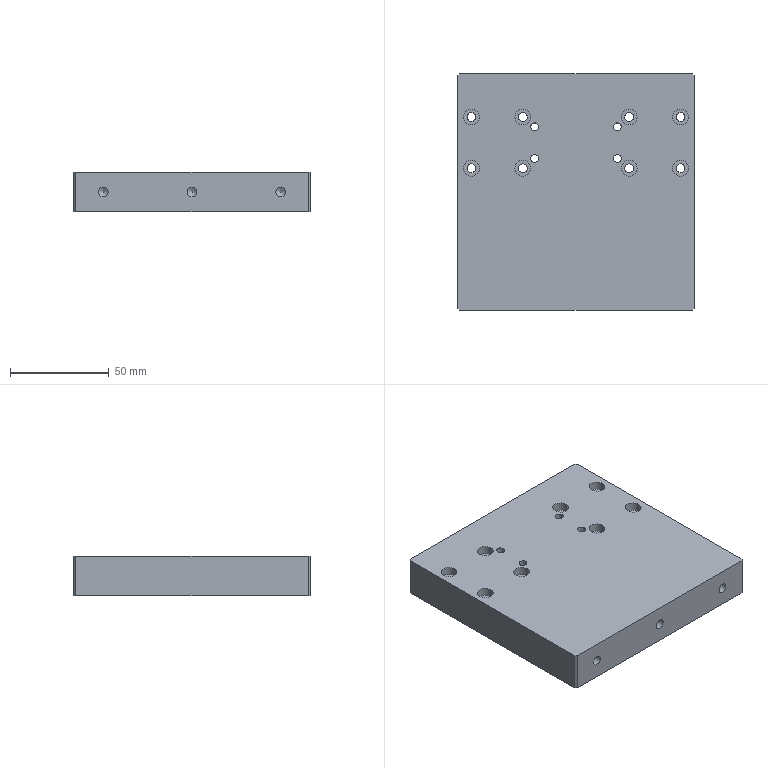CAM job | NX | 3-axis milling, drilling | part box 120 x 120 x 20 mm | stock box 125 x 120 x 25 mm
Tools:
number,name,description,diameter,corner_radius,flute_length,length,flutes
4,D4,平底铣刀-粗,4.0,0.0,25.0,75.0,2
9,D10,平底铣刀-粗,10.0,0.0,35.0,75.0,2
11,D4-J,平底铣刀-精,4.0,0.0,50.0,75.0,2
10,D10-J,平底铣刀-精,10.0,0.0,35.0,75.0,2
1,D80R0.8飞刀,圆鼻刀-粗,80.0,0.8,50.0,75.0,2
1,D80R0.8飞刀-J,圆鼻刀-精,80.0,0.8,50.0,75.0,2
2,D6倒角刀,倒角刀,6.0,0.0,3.0,25.0,2
18,D4铰刀,Drilling Tool,4.0,0.0,75.0,100.0,6
11,ZT4.5,钻头,4.5,0.0,35.0,50.0,2
17,ZT3.9,Drilling Tool,3.9,0.0,35.0,50.0,2
Operations:
program,operation,operation_type,tool,method,geometry_group,spindle_rpm,surface_speed,feed_per_tooth,feed_cut,feed_plunge,cut_length_mm,path_length_mm,cut_time_min,machine_time_min
B,BOTTOM_WALL_FLY_ROUGH_COPY,VolumeBased25DMillingOperation,D80R0.8飞刀,LAYERED_ROUGH-DEPTHK-STEPG,W-B,2800.0,703.696,0.5357,3000.0,100.0,4377.187,4987.758,1.459,1.52
B,BOTTOM_WALL_FLY_FINISH_COPY,VolumeBased25DMillingOperation,D80R0.8飞刀-J,SIDE_FINISH-DEPTHK-STEPG,W-B,4000.0,1005.28,0.125,1000.0,100.0,679.584,775.584,0.6796,0.6892
B,DRILL_CHAMFER_2,Operation,D6倒角刀,METHOD,W-B,8000.0,150.796,0.0625,1000.0,0.0,21.2,226.065,0.0212,0.0417
B,DRILL_CHAMFER_3,Operation,D6倒角刀,METHOD,W-B,8000.0,150.796,0.0625,1000.0,0.0,44.4,420.918,0.0444,0.0821
B,PLANAR_DEBURR_6X45L_COPY,SurfaceContour,D6倒角刀,CLIMB_CHAMFER-DEPTH0-STEPG,W-B,6500.0,122.519,0.1154,1500.0,100.0,622.57,1155.001,0.415,0.4683
A,TOP_FACE,FaceMilling,D80R0.8飞刀,SIDE_FINISH-DEPTHK-STEPG,W-A,4500.0,1385.0,0.1667,1500.0,100.0,714.0,810.0,0.476,0.4856
A,PROFILE_ROUGH_2,VolumeBased25DMillingOperation,D10,METHOD,W-A,8000.0,251.327,0.375,6000.0,80.0,13763.445,13881.945,2.294,2.306
A,SPOT,Operation,D6倒角刀,METHOD,W-A,8000.0,150.796,0.1562,2500.0,0.0,30.0,392.311,0.012,0.0482
A,DRILL,Operation,ZT3.9,METHOD,W-A,3800.0,46.558,0.0395,300.0,0.0,100.503,378.081,0.335,0.3628
A,DRILL_2,Operation,ZT4.5,METHOD,W-A,3800.0,53.721,0.0395,300.0,0.0,186.815,690.756,0.6227,0.6731
A,HOLE_ROUGH_1,CylinderMilling,D4,METHOD,W-A,8000.0,100.531,0.1125,1800.0,100.0,1448.799,2491.599,0.8049,0.9092
A,HOLE_SIDE_1,CylinderMilling,D4-J,METHOD,W-A,8000.0,100.531,0.0375,600.0,100.0,140.141,1220.541,0.2336,0.3416
A,SOLIDS_ONLY,SurfaceContour,D6倒角刀,METHOD,W-A,8000.0,150.796,0.1875,3000.0,100.0,494.959,590.76,0.165,0.1746
A,DRILL_CHAMFER_1,Operation,D6倒角刀,METHOD,W-A,8000.0,150.796,0.0094,150.0,0.0,21.2,226.065,0.1413,0.1618
A,MILL_CHAMFER_1,PlanarMilling,D6倒角刀,METHOD,W-A,8000.0,150.796,0.0375,600.0,100.0,167.71,1202.162,0.2795,0.383
A,REAM_HOLE,Operation,D4铰刀,METHOD,W-A,500.0,6.283,0.0333,100.0,0.0,88.0,353.074,0.88,0.9065
A,PROFILE_SEMI_2,VolumeBased25DMillingOperation,D10-J,METHOD,W-A,9000.0,169.646,0.0667,1200.0,100.0,1028.062,1288.576,0.8567,0.8828
A,BOTTOM_WALL_FINISH_SIDE-MID_COPY,VolumeBased25DMillingOperation,D10-J,SIDE_FINISH-DEPTHK-STEPG,W-A,8000.0,251.32,0.0625,1000.0,100.0,544.45,1036.562,0.5444,0.5937